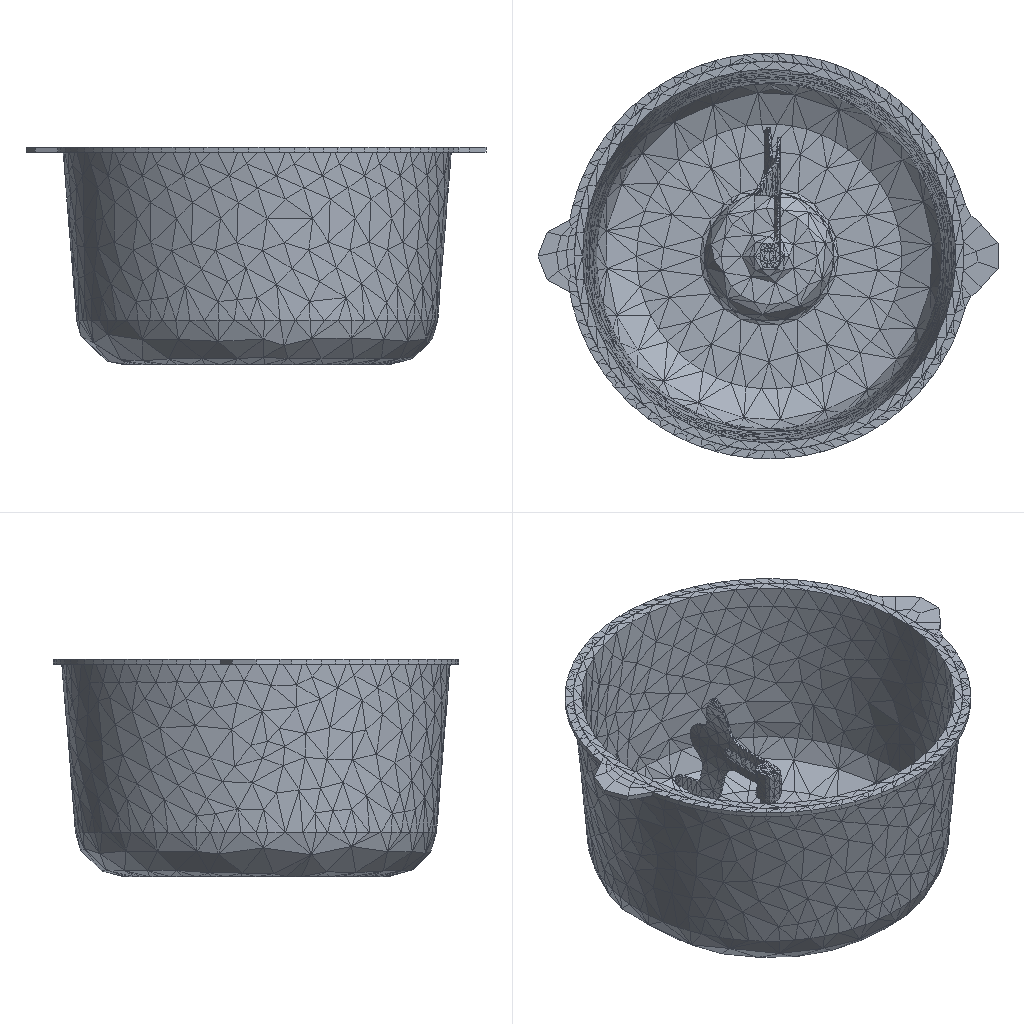Simulation study | ansys workbench
Set-up summary:
category,name,step,type,value,unit,region
solver,ansys_mapdl
solver,version,,,22.1
units,MPA,,stated
analysis,deck,,static,static
load_step,requested,,,1
analysis,nlgeom,,,False
mesh,nodes,,,13115
mesh,elements,,,6964
element_type,ANSYS 186 (type 1),,solid,207
element_type,ANSYS 187 (type 2),,solid,3736
element_type,ANSYS 187 (type 3),,solid,649
element_type,ANSYS 187 (type 4),,solid,942
element_type,ANSYS 187 (type 5),,solid,36
element_type,ANSYS 174 (type 6),,contact,263
element_type,ANSYS 170 (type 7),,target,263
element_type,ANSYS 174 (type 8),,contact,44
element_type,ANSYS 170 (type 9),,target,44
element_type,ANSYS 174 (type 10),,contact,221
element_type,ANSYS 170 (type 11),,target,221
element_type,ANSYS 174 (type 12),,contact,90
element_type,ANSYS 170 (type 13),,target,90
element_type,ANSYS 174 (type 14),,contact,158
element_type,ANSYS 170 (type 15),,target,0
load,load commands in deck,,count,3
bc,support commands in deck,,count,1
named_set,_FIXEDSU,,component
material,1,,in results
material,2,,in results
material,3,,in results
material,4,,in results
material,5,,in results
check,setup vs results,,match,results also hold 1 node(s) and 1 element(s) the deck makes with ['EN']; those were not compared
Ansys APDL input file, long lists of numbers shortened:
/batch
/config,noeldb,1     ! force off writing results to database
*get,_wallstrt,active,,time,wall
! ANSYS input file written by Workbench version 2022 R1
! File used for geometry attach: F:\ansys（分析文件汇总)\搅拌锅有限元分析\实验.stp
/title,wbnew--____ (B5)
! ****** Begin Custom Load Command Snippet ******
/COM, ACT Extensions:
/COM,     LSDYNA, 2021.1
/COM,
! ****** End   Custom Load Command Snippet ******
*DIM,_wb_ProjectScratch_dir,string,248
_wb_ProjectScratch_dir(1) = 'C:\Users\Administrator\AppData\Local\Temp\WB_Administrator_25620_2\_ProjectScratch\Scr1057\'
*DIM,_wb_SolverFiles_dir,string,248
_wb_SolverFiles_dir(1) = 'C:\Users\Administrator\AppData\Local\Temp\WB_Administrator_25620_2\wbnew_files\dp0\SYS\MECH\'
*DIM,_wb_userfiles_dir,string,248
_wb_userfiles_dir(1) = 'C:\Users\Administrator\AppData\Local\Temp\WB_Administrator_25620_2\wbnew_files\user_files\'
/com,--- Data in consistent NMM units. See Solving Units in the help system for more information.
/units,MPA
/nopr
/wb,file,start              !  signify a WB generated input file
/prep7
! Turn off shape checking because checks already performed inside WB mesher.
! See help system for more information.
SHPP,OFF,,NOWARN
/nolist
etcon,set             ! allow ANSYS to choose best KEYOP's for 180x elements, resets any applicable keyopt to MAPDL defaults
/com,*********** Nodes for the whole assembly ***********
nblock,3,,14425
(1i9,3e20.9e3)
        1    -1.679881389E+01     1.287663067E+01     5.951140611E+01
! (13113 more lines like these left out)
-1
/com,*********** Nodes for all Remote Points ***********
nblock,3
(1i9,3e20.9e3)
    13115    -1.852799638E+01     1.843413194E+01     6.278717582E+01
-1
/wb,elem,start            !  set before creation of elements
/com,*********** Elements for Body 1 "___|___" ***********
et,1,186
keyo,1,2,1          ! set full integration on SOLID186
eblock,19,solid,,207
(19i9)
        1        1        1        1        0        0        0        0       20        0       37      160      566      567      725      229      455      457      415
! (413 more lines like these left out)
-1
/com,*********** Elements for Body 2 "___|___[2]" ***********
et,2,187
eblock,19,solid,,3736
(19i9)
        2        2        2        2        0        0        0        0       10        0     1835     5744     6715     6668     6013     8506    12850     8505     8504
! (7471 more lines like these left out)
-1
/com,*********** Elements for Body 3 "___|___" ***********
et,3,187
eblock,19,solid,,649
(19i9)
        3        3        3        3        0        0        0        0       10        0      244     2239     2290     2270     2271     3241     3356     3234     3235
! (1297 more lines like these left out)
-1
/com,*********** Elements for Body 4 "___|___" ***********
et,4,187
eblock,19,solid,,942
(19i9)
        4        4        4        4        0        0        0        0       10        0      893     3526     3779     3719     3776     4542     5379     4538     4541
! (1883 more lines like these left out)
-1
/com,*********** Elements for Body 5 "___|WLD1" ***********
et,5,187
eblock,19,solid,,36
(19i9)
        5        5        5        5        0        0        0        0       10        0        1        5       34       16       17       61      108       59       60
! (71 more lines like these left out)
-1
/wb,elem,end               !  done creating elements
/com,*********** Send User Defined Coordinate System(s) ***********
csys,0
toffst,273.15,  ! Temperature offset from absolute zero
/com,*********** Set Reference Temperature ***********
tref,22.
/wb,mat,start              !  starting to send materials
/com,*********** Send Materials ***********
Temperature = 'TEMP' ! Temperature
MP,DENS,1,1.08e-09,	! tonne mm^-3
MP,ALPX,1,1.2e-05,	! C^-1
MP,C,1,434000000,	! mm^2 s^-2 C^-1
MP,KXX,1,60.5,	! tonne mm s^-3 C^-1
MP,RSVX,1,0.00017,	! ohm mm
MP,EX,1,2000,	! tonne s^-2 mm^-1
MP,NUXY,1,0.35,
MP,MURX,1,10000,
Temperature = 'TEMP' ! Temperature
MP,DENS,2,1.08e-09,	! tonne mm^-3
MP,ALPX,2,1.2e-05,	! C^-1
MP,C,2,434000000,	! mm^2 s^-2 C^-1
MP,KXX,2,60.5,	! tonne mm s^-3 C^-1
MP,RSVX,2,0.00017,	! ohm mm
MP,EX,2,2000,	! tonne s^-2 mm^-1
MP,NUXY,2,0.35,
MP,MURX,2,10000,
Temperature = 'TEMP' ! Temperature
MP,DENS,3,7.85e-09,	! tonne mm^-3
MP,ALPX,3,1.2e-05,	! C^-1
MP,C,3,434000000,	! mm^2 s^-2 C^-1
MP,KXX,3,60.5,	! tonne mm s^-3 C^-1
MP,RSVX,3,0.00017,	! ohm mm
MP,EX,3,200000,	! tonne s^-2 mm^-1
MP,NUXY,3,0.3,
MP,MURX,3,10000,
Temperature = 'TEMP' ! Temperature
MP,DENS,4,7.85e-09,	! tonne mm^-3
MP,ALPX,4,1.2e-05,	! C^-1
MP,C,4,434000000,	! mm^2 s^-2 C^-1
MP,KXX,4,60.5,	! tonne mm s^-3 C^-1
MP,RSVX,4,0.00017,	! ohm mm
MP,EX,4,200000,	! tonne s^-2 mm^-1
MP,NUXY,4,0.3,
MP,MURX,4,10000,
Temperature = 'TEMP' ! Temperature
MP,DENS,5,7.85e-09,	! tonne mm^-3
MP,ALPX,5,1.2e-05,	! C^-1
MP,C,5,434000000,	! mm^2 s^-2 C^-1
MP,KXX,5,60.5,	! tonne mm s^-3 C^-1
MP,RSVX,5,0.00017,	! ohm mm
MP,EX,5,200000,	! tonne s^-2 mm^-1
MP,NUXY,5,0.3,
MP,MURX,5,10000,
/wb,mat,end                !  done sending materials
!************************* Model Summary ********************
!___|___,	ABS,	matid,	1
!___|___[2],	ABS,	matid,	2
!___|___,	45钢,	matid,	3
!___|___,	304,	matid,	4
!___|WLD1,	304,	matid,	5
!************************* End Model Summary ********************
! get the diagonal of the bounding box. Needed later for other things
*get,_xmin,node,,mnloc,x
*get,_ymin,node,,mnloc,y
*get,_zmin,node,,mnloc,z
*get,_xmax,node,,mxloc,x
*get,_ymax,node,,mxloc,y
*get,_zmax,node,,mxloc,z
_ASMDIAG=(_xmax-_xmin)*(_xmax-_xmin)+(_ymax-_ymin)*(_ymax-_ymin)+(_zmax-_zmin)*(_zmax-_zmin)
_ASMDIAG=SQRT(_ASMDIAG)
/wb,contact,start          !  starting to send contact
/com,*********** Create Contact "接触区域" ***********
/com,            Real Constant Set For Above Contact Is 7 & 6
*set,tid,7
*set,cid,6
r,tid
r,cid
et,tid,170
et,cid,174
eblock,10,,,161
(15i9)
    10056        7        7        7        0      260      570      569      419     1109     1881     1542     1108
! (160 more lines like these left out)
-1
eblock,10,,,161
(15i9)
    10217        6        6        6        0      260      570      569      419     1109     1881     1542     1108
! (160 more lines like these left out)
-1
eblock,10,,,102
(15i9)
    10378        6        7        6        0     6447     5540     5541     5541     7133     7128     5541     7138
! (101 more lines like these left out)
-1
eblock,10,,,102
(15i9)
    10480        7        6        7        0     6447     5540     5541     5541     7133     7128     5541     7138
! (101 more lines like these left out)
-1
keyo,cid,8,2               ! auto create asymmetric contact (from Program Controlled setting)
keyo,cid,10,0              ! adjust contact stiffness each NR iteration (from Program Controlled setting)
keyo,cid,12,5              ! bonded always
keyo,cid,18,1              ! small sliding turned on by application
keyo,cid,2,0               ! augmented Lagrange (from Program Controlled setting)
keyo,cid,4,0               ! on Gauss point (from Program Controlled setting)
keyo,cid,9,1               ! ignore initial gaps/penetration
keyo,cid,7,0               ! No Prediction
rmod,tid,3,10.      ! FKN
rmod,tid,5,0.       ! ICONT
rmod,tid,6,0.       ! PINB
rmod,tid,10,0.      ! CNOF
rmod,tid,12,0.      ! FKT
rmod,tid,36,43      ! WB DSID
rmod,cid,3,10.      ! FKN
rmod,cid,5,0.       ! ICONT
rmod,cid,6,0.       ! PINB
rmod,cid,10,0.      ! CNOF
rmod,cid,12,0.      ! FKT
rmod,cid,36,43      ! WB DSID
/com,*********** Create Contact "接触区域 2" ***********
/com,            Real Constant Set For Above Contact Is 9 & 8
*set,tid,9
*set,cid,8
r,tid
r,cid
et,tid,170
et,cid,174
eblock,10,,,14
(15i9)
    10582        9        9        9        0     5812     5821     5822     5822     9065     9117     5822     9066
! (13 more lines like these left out)
-1
eblock,10,,,14
(15i9)
    10596        8        8        8        0     5812     5821     5822     5822     9065     9117     5822     9066
! (13 more lines like these left out)
-1
eblock,10,,,30
(15i9)
    10610        8        9        8        0     2057     2059     2060     2060     2314     2325     2060     2315
! (29 more lines like these left out)
-1
eblock,10,,,30
(15i9)
    10640        9        8        9        0     2057     2059     2060     2060     2314     2325     2060     2315
! (29 more lines like these left out)
-1
keyo,cid,8,2               ! auto create asymmetric contact (from Program Controlled setting)
keyo,cid,10,0              ! adjust contact stiffness each NR iteration (from Program Controlled setting)
keyo,cid,12,5              ! bonded always
keyo,cid,18,1              ! small sliding turned on by application
keyo,cid,2,0               ! augmented Lagrange (from Program Controlled setting)
keyo,cid,4,0               ! on Gauss point (from Program Controlled setting)
keyo,cid,9,1               ! ignore initial gaps/penetration
keyo,cid,7,0               ! No Prediction
rmod,tid,3,10.      ! FKN
rmod,tid,5,0.       ! ICONT
rmod,tid,6,0.       ! PINB
rmod,tid,10,0.      ! CNOF
rmod,tid,12,0.      ! FKT
rmod,tid,36,46      ! WB DSID
rmod,cid,3,10.      ! FKN
rmod,cid,5,0.       ! ICONT
rmod,cid,6,0.       ! PINB
rmod,cid,10,0.      ! CNOF
rmod,cid,12,0.      ! FKT
rmod,cid,36,46      ! WB DSID
/com,*********** Create Contact "接触区域 3" ***********
/com,            Real Constant Set For Above Contact Is 11 & 10
*set,tid,11
*set,cid,10
r,tid
r,cid
et,tid,170
et,cid,174
eblock,10,,,141
(15i9)
    10670       11       11       11        0     2225     2149     2253     2253     2772     2775     2253     3183
! (140 more lines like these left out)
-1
eblock,10,,,141
(15i9)
    10811       10       10       10        0     2225     2149     2253     2253     2772     2775     2253     3183
! (140 more lines like these left out)
-1
eblock,10,,,80
(15i9)
    10952       10       11       10        0     3491     3501     3665     3665     4324     4393     3665     4330
! (79 more lines like these left out)
-1
eblock,10,,,80
(15i9)
    11032       11       10       11        0     3491     3501     3665     3665     4324     4393     3665     4330
! (79 more lines like these left out)
-1
keyo,cid,8,2               ! auto create asymmetric contact (from Program Controlled setting)
keyo,cid,10,0              ! adjust contact stiffness each NR iteration (from Program Controlled setting)
keyo,cid,12,5              ! bonded always
keyo,cid,18,1              ! small sliding turned on by application
keyo,cid,2,0               ! augmented Lagrange (from Program Controlled setting)
keyo,cid,4,0               ! on Gauss point (from Program Controlled setting)
keyo,cid,9,1               ! ignore initial gaps/penetration
keyo,cid,7,0               ! No Prediction
rmod,tid,3,10.      ! FKN
rmod,tid,5,0.       ! ICONT
rmod,tid,6,0.       ! PINB
rmod,tid,10,0.      ! CNOF
rmod,tid,12,0.      ! FKT
rmod,tid,36,49      ! WB DSID
rmod,cid,3,10.      ! FKN
rmod,cid,5,0.       ! ICONT
rmod,cid,6,0.       ! PINB
rmod,cid,10,0.      ! CNOF
rmod,cid,12,0.      ! FKT
rmod,cid,36,49      ! WB DSID
/com,*********** Create Contact "接触区域 4" ***********
/com,            Real Constant Set For Above Contact Is 13 & 12
*set,tid,13
*set,cid,12
r,tid
r,cid
et,tid,170
et,cid,174
eblock,10,,,60
(15i9)
    11112       13       13       13        0     3637     3724     3723     3723     5017     5381     3723     5016
! (59 more lines like these left out)
-1
eblock,10,,,60
(15i9)
    11172       12       12       12        0     3637     3724     3723     3723     5017     5381     3723     5016
! (59 more lines like these left out)
-1
eblock,10,,,30
(15i9)
    11232       12       13       12        0        4       17        5        5       54       60        5       53
! (29 more lines like these left out)
-1
eblock,10,,,30
(15i9)
    11262       13       12       13        0        4       17        5        5       54       60        5       53
! (29 more lines like these left out)
-1
keyo,cid,8,2               ! auto create asymmetric contact (from Program Controlled setting)
keyo,cid,10,0              ! adjust contact stiffness each NR iteration (from Program Controlled setting)
keyo,cid,12,5              ! bonded always
keyo,cid,18,1              ! small sliding turned on by application
keyo,cid,2,0               ! augmented Lagrange (from Program Controlled setting)
keyo,cid,4,0               ! on Gauss point (from Program Controlled setting)
keyo,cid,9,1               ! ignore initial gaps/penetration
keyo,cid,7,0               ! No Prediction
rmod,tid,3,10.      ! FKN
rmod,tid,5,0.       ! ICONT
rmod,tid,6,0.       ! PINB
rmod,tid,10,0.      ! CNOF
rmod,tid,12,0.      ! FKT
rmod,tid,36,52      ! WB DSID
rmod,cid,3,10.      ! FKN
rmod,cid,5,0.       ! ICONT
rmod,cid,6,0.       ! PINB
rmod,cid,10,0.      ! CNOF
rmod,cid,12,0.      ! FKT
rmod,cid,36,52      ! WB DSID
nsel,all
esel,all
/wb,contact,end            !  done creating contacts
/golist
/wb,load,start             !  starting to send loads
/com,*********** Fixed Supports ***********
CMBLOCK,_FIXEDSU,NODE,      439
(8i10)
      2053      2054      2055      2056      2057      2058      2059      2060
! (54 more lines like these left out)
cmsel,s,_FIXEDSU
d,all,all
nsel,all
/com,*********** Create Remote Point "内部远程点" ***********
! -------- Remote Point Used by "力矩" --------
*set,tid,15
*set,cid,14
et,cid,174
et,tid,170
keyo,tid,2,1               ! Don't fix the pilot node
keyo,tid,4,111111
keyo,cid,12,5              ! Bonded Contact
keyo,cid,4,1               ! Deformable RBE3 style load
keyo,cid,2,2               ! MPC style contact
eblock,10,,,158
(15i9)
    11292       14       14       14        0     3637     3724     3723     3723     5017     5381     3723     5016
! (157 more lines like these left out)
-1
*set,_npilot,13115
_npilot61=_npilot
type,tid
mat ,cid
real,cid
tshape,pilo
en,11450,_npilot
tshape
/com,*********** Construct Moment Using Remote Attachment ***********
/gst,on,on
fini
*get,_numnode,node,0,count
*get,_numelem,elem,0,count
*get, _MAXELEMNUM, elem, 0, NUM, MAX
*get, _MAXNODENUM, node, 0, NUM, MAX
*get, _MAXELEMTYPE, etyp, 0, NUM, MAX
*get, _MAXREALCONST, real, 0, NUM, MAX
/go
/wb,load,end               !  done creating loads
/com,--- Number of total nodes = %_numnode%
/com,--- Number of contact elements = 1394
/com,--- Number of spring elements = 0
/com,--- Number of bearing elements = 0
/com,--- Number of solid elements = 5570
/com,--- Number of condensed parts = 0
/com,--- Number of total elements = %_numelem%
*get,_wallbsol,active,,time,wall
/com,****************************************************************************
/com,*************************    SOLUTION       ********************************
/com,****************************************************************************
/solu
antype,0                   ! static analysis
_thickRatio=  0     ! Ratio of thick parts in the model
eqsl,sparse,,,,,1
cntr,print,1               ! print out contact info and also make no initial contact an error
dmpoption,emat,no             ! Don't combine emat file for DANSYS
dmpoption,esav,no             ! Don't combine esav file for DANSYS
nldiag,cont,iter           ! print out contact info each equilibrium iteration
rescontrol,,none                 ! Do not keep any restart files
/com,****************************************************
/com,******************* SOLVE FOR LS 1 OF 1 ****************
nsel,s,node,,13115
f,all,mx,0.
f,all,my,0.
f,all,mz,637.
nsel,all
/nopr
/gopr
nsub,1,1,1
time,1.
outres,erase
outres,all,none
outres,nsol,all,
outres,rsol,all
outres,eangl,all
outres,etmp,all
outres,veng,all
outres,strs,all,
outres,epel,all,
outres,eppl,all,
outres,cont,all,
! *********** WB SOLVE COMMAND ***********
! check interactive state
*get,ANSINTER_,active,,int
*if,ANSINTER_,ne,0,then
/eof
*endif
solve
/com *************** Write FE CONNECTORS *********
CEWRITE,file,ce,,INTE
/com,****************************************************
/com,*************** FINISHED SOLVE FOR LS 1 *************
*get,_wallasol,active,,time,wall
/nopr
*get,_numnode,node,0,count
*get,_numelem,elem,0,count
*get, _MAXELEMNUM, elem, 0, NUM, MAX
*get, _MAXNODENUM, node, 0, NUM, MAX,,,INTERNAL
*get, _MAXELEMTYPE, etyp, 0, NUM, MAX
*get, _MAXREALCONST, real, 0, NUM, MAX
/gopr
/post1
xmlo,ENCODING,ISO-8859-1
xmlo,parm
/xml,parm,xml
fini
/gopr
*get,_walldone,active,,time,wall
_preptime=(_wallbsol-_wallstrt)*3600
_solvtime=(_wallasol-_wallbsol)*3600
_posttime=(_walldone-_wallasol)*3600
_totaltim=(_walldone-_wallstrt)*3600
*get,_dlbratio,active,0,solu,dlbr
*get,_combtime,active,0,solu,comb
*get,_ssmode,active,0,solu,ssmm
*get,_ndofs,active,0,solu,ndof
*get,_sol_end_time,active,0,set,time
*if,_sol_end_time,eq,1.,then
/fclean				!clean distributed files
*endif
/com,--- Total number of nodes = %_numnode%
/com,--- Total number of elements = %_numelem%
/com,--- Element load balance ratio = %_dlbratio%
/com,--- Time to combine distributed files = %_combtime%
/com,--- Sparse memory mode = %_ssmode%
/com,--- Number of DOF = %_ndofs%
/wb,file,end               ! done with WB generated input
Results summary:
result,analysis,,,static
result,last_loadstep,,,1
result,primary field,,,displacement
result,reaction total,1,FX,0.0,N
result,reaction total,1,FY,-0.0,N
result,reaction total,1,FZ,0.0,N
result,mass,,,0.000787,"NMM: mm, ton, N, s, mV, mA, degC"